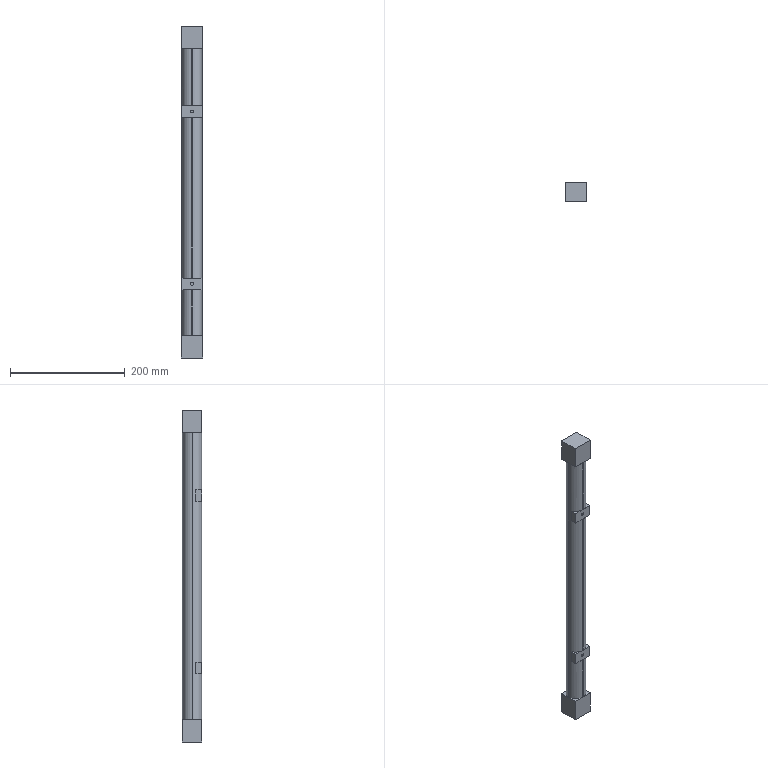Part | STEP file | LED lamp for distribution cabinet QELTS-500-220 | 1 solid | 50 faces | box 37 x 33.2 x 578 mm | volume 564522 mm3 | plane 43 | cylinder 7 | commonest cylinder face diameters 4.2 x4 33.2 x3